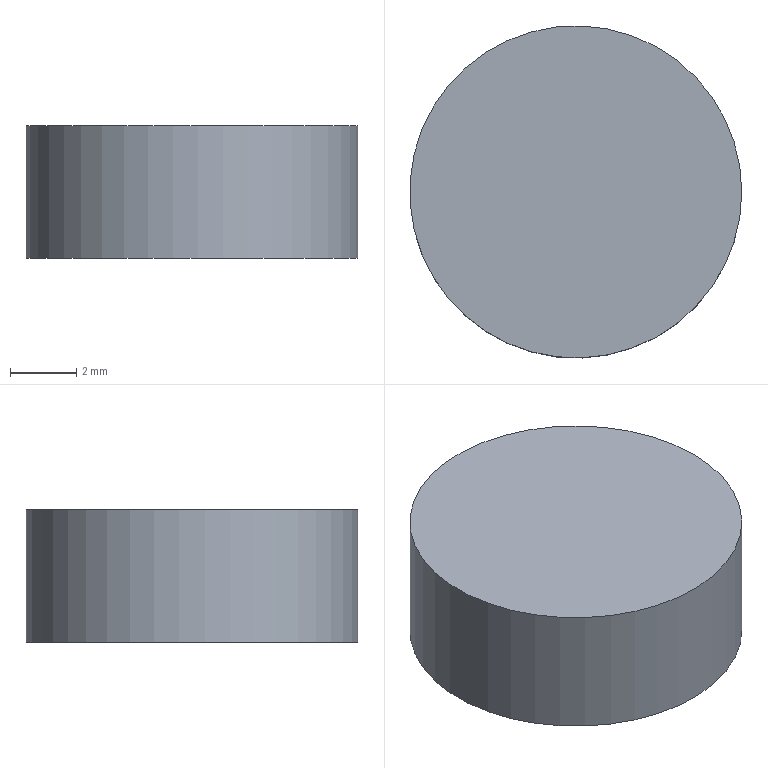Part | NX | features DATUM_CSYS 2, EXTRUDE 1, SKETCH 1 | 1 solid | 3 faces | box 10 x 10 x 4 mm | volume 314.159 mm3 | plane 2 | cylinder 1 | commonest cylinder face diameters 10 x1
STEP:
#1=CARTESIAN_POINT('',(5.,0.,4.));
#2=VERTEX_POINT('',#1);
#3=CARTESIAN_POINT('',(0.,0.,4.));
#4=DIRECTION('',(0.,0.,1.));
#5=DIRECTION('',(1.,0.,0.));
#6=AXIS2_PLACEMENT_3D('',#3,#4,#5);
#7=CIRCLE('',#6,5.);
#8=EDGE_CURVE('',#2,#2,#7,.T.);
#9=ORIENTED_EDGE('',*,*,#8,.F.);
#10=EDGE_LOOP('',(#9));
#11=FACE_BOUND('',#10,.T.);
#12=CARTESIAN_POINT('',(5.,0.,0.));
#13=VERTEX_POINT('',#12);
#14=CARTESIAN_POINT('',(0.,0.,0.));
#15=DIRECTION('',(0.,0.,1.));
#16=DIRECTION('',(1.,0.,0.));
#17=AXIS2_PLACEMENT_3D('',#14,#15,#16);
#18=CIRCLE('',#17,5.);
#19=EDGE_CURVE('',#13,#13,#18,.T.);
#20=ORIENTED_EDGE('',*,*,#19,.T.);
#21=EDGE_LOOP('',(#20));
#22=FACE_BOUND('',#21,.T.);
#23=CARTESIAN_POINT('',(0.,0.,4.));
#24=DIRECTION('',(0.,0.,-1.));
#25=DIRECTION('',(-1.,0.,0.));
#26=AXIS2_PLACEMENT_3D('',#23,#24,#25);
#27=CYLINDRICAL_SURFACE('',#26,5.);
#28=ADVANCED_FACE('',(#11,#22),#27,.T.);
#29=ORIENTED_EDGE('',*,*,#8,.T.);
#30=EDGE_LOOP('',(#29));
#31=FACE_BOUND('',#30,.T.);
#32=CARTESIAN_POINT('',(0.,0.,4.));
#33=DIRECTION('',(0.,0.,1.));
#34=DIRECTION('',(1.,0.,0.));
#35=AXIS2_PLACEMENT_3D('',#32,#33,#34);
#36=PLANE('',#35);
#37=ADVANCED_FACE('',(#31),#36,.T.);
#38=ORIENTED_EDGE('',*,*,#19,.F.);
#39=EDGE_LOOP('',(#38));
#40=FACE_BOUND('',#39,.T.);
#41=CARTESIAN_POINT('',(0.,0.,0.));
#42=DIRECTION('',(0.,0.,1.));
#43=DIRECTION('',(1.,0.,0.));
#44=AXIS2_PLACEMENT_3D('',#41,#42,#43);
#45=PLANE('',#44);
#46=ADVANCED_FACE('',(#40),#45,.F.);
#47=CLOSED_SHELL('',(#28,#37,#46));
#48=MANIFOLD_SOLID_BREP('',#47);
#49=(LENGTH_UNIT()NAMED_UNIT(*)SI_UNIT(.MILLI.,.METRE.));
#50=UNCERTAINTY_MEASURE_WITH_UNIT(LENGTH_MEASURE(0.00001),#49,'','');
#51=(NAMED_UNIT(*)PLANE_ANGLE_UNIT()SI_UNIT($,.RADIAN.));
#52=(NAMED_UNIT(*)SI_UNIT($,.STERADIAN.)SOLID_ANGLE_UNIT());
#53=(GEOMETRIC_REPRESENTATION_CONTEXT(3)GLOBAL_UNCERTAINTY_ASSIGNED_CONTEXT((#50))GLOBAL_UNIT_ASSIGNED_CONTEXT((#49,#51,#52))REPRESENTATION_CONTEXT('',''));
#54=ADVANCED_BREP_SHAPE_REPRESENTATION('',(#48),#53);